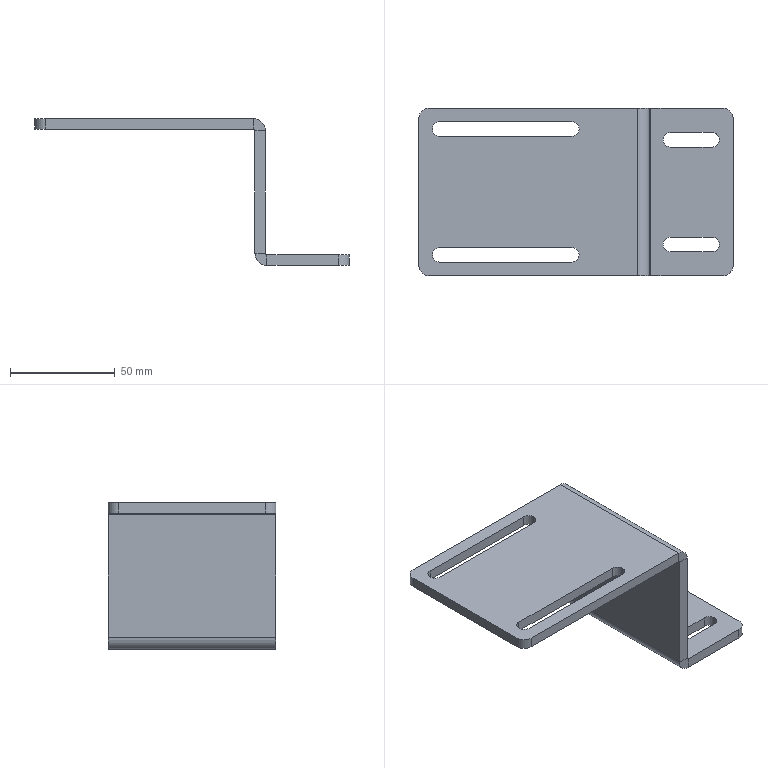Part | SolidWorks | features BaseBody 1 | 1 solid | 46 faces | box 150 x 80 x 70 mm | volume 78202 mm3 | plane 26 | cylinder 20 | commonest cylinder face diameters 7 x12 10 x4 1.473 x2 11.473 x2
STEP:
#1=CARTESIAN_POINT('',(110.,-21.5,-70.));
#2=VERTEX_POINT('',#1);
#3=CARTESIAN_POINT('',(113.5,-25.,-70.));
#4=VERTEX_POINT('',#3);
#5=CARTESIAN_POINT('',(110.,-25.,-70.));
#6=DIRECTION('',(0.,0.,-1.));
#7=DIRECTION('',(-1.,0.,0.));
#8=AXIS2_PLACEMENT_3D('',#5,#6,#7);
#9=CIRCLE('',#8,3.5);
#10=EDGE_CURVE('',#2,#4,#9,.T.);
#11=ORIENTED_EDGE('',*,*,#10,.T.);
#12=CARTESIAN_POINT('',(113.5,-25.,-65.));
#13=VERTEX_POINT('',#12);
#14=CARTESIAN_POINT('',(113.5,-25.,-75.));
#15=DIRECTION('',(0.,0.,1.));
#16=VECTOR('',#15,1000.);
#17=LINE('',#14,#16);
#18=EDGE_CURVE('',#4,#13,#17,.T.);
#19=ORIENTED_EDGE('',*,*,#18,.T.);
#20=CARTESIAN_POINT('',(110.,-21.5,-65.));
#21=VERTEX_POINT('',#20);
#22=CARTESIAN_POINT('',(110.,-25.,-65.));
#23=DIRECTION('',(0.,0.,1.));
#24=DIRECTION('',(1.,0.,0.));
#25=AXIS2_PLACEMENT_3D('',#22,#23,#24);
#26=CIRCLE('',#25,3.5);
#27=EDGE_CURVE('',#13,#21,#26,.T.);
#28=ORIENTED_EDGE('',*,*,#27,.T.);
#29=CARTESIAN_POINT('',(110.,-21.5,-75.));
#30=DIRECTION('',(0.,0.,1.));
#31=VECTOR('',#30,1000.);
#32=LINE('',#29,#31);
#33=EDGE_CURVE('',#2,#21,#32,.T.);
#34=ORIENTED_EDGE('',*,*,#33,.F.);
#35=EDGE_LOOP('',(#11,#19,#28,#34));
#36=FACE_OUTER_BOUND('',#35,.T.);
#37=CARTESIAN_POINT('',(110.,-25.,-75.));
#38=DIRECTION('',(0.,0.,1.));
#39=DIRECTION('',(1.,0.,0.));
#40=AXIS2_PLACEMENT_3D('',#37,#38,#39);
#41=CYLINDRICAL_SURFACE('',#40,3.5);
#42=ADVANCED_FACE('',(#36),#41,.F.);
#43=CARTESIAN_POINT('',(110.,28.5,-70.));
#44=VERTEX_POINT('',#43);
#45=CARTESIAN_POINT('',(113.5,25.,-70.));
#46=VERTEX_POINT('',#45);
#47=CARTESIAN_POINT('',(110.,25.,-70.));
#48=DIRECTION('',(0.,0.,-1.));
#49=DIRECTION('',(-1.,0.,0.));
#50=AXIS2_PLACEMENT_3D('',#47,#48,#49);
#51=CIRCLE('',#50,3.5);
#52=EDGE_CURVE('',#44,#46,#51,.T.);
#53=ORIENTED_EDGE('',*,*,#52,.T.);
#54=CARTESIAN_POINT('',(113.5,25.,-65.));
#55=VERTEX_POINT('',#54);
#56=CARTESIAN_POINT('',(113.5,25.,-75.));
#57=DIRECTION('',(0.,0.,1.));
#58=VECTOR('',#57,1000.);
#59=LINE('',#56,#58);
#60=EDGE_CURVE('',#46,#55,#59,.T.);
#61=ORIENTED_EDGE('',*,*,#60,.T.);
#62=CARTESIAN_POINT('',(110.,28.5,-65.));
#63=VERTEX_POINT('',#62);
#64=CARTESIAN_POINT('',(110.,25.,-65.));
#65=DIRECTION('',(0.,0.,1.));
#66=DIRECTION('',(1.,0.,0.));
#67=AXIS2_PLACEMENT_3D('',#64,#65,#66);
#68=CIRCLE('',#67,3.5);
#69=EDGE_CURVE('',#55,#63,#68,.T.);
#70=ORIENTED_EDGE('',*,*,#69,.T.);
#71=CARTESIAN_POINT('',(110.,28.5,-75.));
#72=DIRECTION('',(0.,0.,1.));
#73=VECTOR('',#72,1000.);
#74=LINE('',#71,#73);
#75=EDGE_CURVE('',#44,#63,#74,.T.);
#76=ORIENTED_EDGE('',*,*,#75,.F.);
#77=EDGE_LOOP('',(#53,#61,#70,#76));
#78=FACE_OUTER_BOUND('',#77,.T.);
#79=CARTESIAN_POINT('',(110.,25.,-75.));
#80=DIRECTION('',(0.,0.,1.));
#81=DIRECTION('',(1.,0.,0.));
#82=AXIS2_PLACEMENT_3D('',#79,#80,#81);
#83=CYLINDRICAL_SURFACE('',#82,3.5);
#84=ADVANCED_FACE('',(#78),#83,.F.);
#85=CARTESIAN_POINT('',(46.5,-30.,-5.));
#86=VERTEX_POINT('',#85);
#87=CARTESIAN_POINT('',(43.,-26.5,-5.));
#88=VERTEX_POINT('',#87);
#89=CARTESIAN_POINT('',(43.,-30.,-5.));
#90=DIRECTION('',(0.,0.,1.));
#91=DIRECTION('',(1.,0.,0.));
#92=AXIS2_PLACEMENT_3D('',#89,#90,#91);
#93=CIRCLE('',#92,3.5);
#94=EDGE_CURVE('',#86,#88,#93,.T.);
#95=ORIENTED_EDGE('',*,*,#94,.F.);
#96=CARTESIAN_POINT('',(46.5,-30.,0.));
#97=VERTEX_POINT('',#96);
#98=CARTESIAN_POINT('',(46.5,-30.,-10.));
#99=DIRECTION('',(0.,0.,1.));
#100=VECTOR('',#99,1000.);
#101=LINE('',#98,#100);
#102=EDGE_CURVE('',#86,#97,#101,.T.);
#103=ORIENTED_EDGE('',*,*,#102,.T.);
#104=CARTESIAN_POINT('',(43.,-26.5,0.));
#105=VERTEX_POINT('',#104);
#106=CARTESIAN_POINT('',(43.,-30.,0.));
#107=DIRECTION('',(0.,0.,1.));
#108=DIRECTION('',(1.,0.,0.));
#109=AXIS2_PLACEMENT_3D('',#106,#107,#108);
#110=CIRCLE('',#109,3.5);
#111=EDGE_CURVE('',#97,#105,#110,.T.);
#112=ORIENTED_EDGE('',*,*,#111,.T.);
#113=CARTESIAN_POINT('',(43.,-26.5,-10.));
#114=DIRECTION('',(0.,0.,1.));
#115=VECTOR('',#114,1000.);
#116=LINE('',#113,#115);
#117=EDGE_CURVE('',#88,#105,#116,.T.);
#118=ORIENTED_EDGE('',*,*,#117,.F.);
#119=EDGE_LOOP('',(#95,#103,#112,#118));
#120=FACE_OUTER_BOUND('',#119,.T.);
#121=CARTESIAN_POINT('',(43.,-30.,-10.));
#122=DIRECTION('',(0.,0.,1.));
#123=DIRECTION('',(1.,0.,0.));
#124=AXIS2_PLACEMENT_3D('',#121,#122,#123);
#125=CYLINDRICAL_SURFACE('',#124,3.5);
#126=ADVANCED_FACE('',(#120),#125,.F.);
#127=CARTESIAN_POINT('',(46.5,30.,-5.));
#128=VERTEX_POINT('',#127);
#129=CARTESIAN_POINT('',(43.,33.5,-5.));
#130=VERTEX_POINT('',#129);
#131=CARTESIAN_POINT('',(43.,30.,-5.));
#132=DIRECTION('',(0.,0.,1.));
#133=DIRECTION('',(1.,0.,0.));
#134=AXIS2_PLACEMENT_3D('',#131,#132,#133);
#135=CIRCLE('',#134,3.5);
#136=EDGE_CURVE('',#128,#130,#135,.T.);
#137=ORIENTED_EDGE('',*,*,#136,.F.);
#138=CARTESIAN_POINT('',(46.5,30.,0.));
#139=VERTEX_POINT('',#138);
#140=CARTESIAN_POINT('',(46.5,30.,-10.));
#141=DIRECTION('',(0.,0.,1.));
#142=VECTOR('',#141,1000.);
#143=LINE('',#140,#142);
#144=EDGE_CURVE('',#128,#139,#143,.T.);
#145=ORIENTED_EDGE('',*,*,#144,.T.);
#146=CARTESIAN_POINT('',(43.,33.5,0.));
#147=VERTEX_POINT('',#146);
#148=CARTESIAN_POINT('',(43.,30.,0.));
#149=DIRECTION('',(0.,0.,1.));
#150=DIRECTION('',(1.,0.,0.));
#151=AXIS2_PLACEMENT_3D('',#148,#149,#150);
#152=CIRCLE('',#151,3.5);
#153=EDGE_CURVE('',#139,#147,#152,.T.);
#154=ORIENTED_EDGE('',*,*,#153,.T.);
#155=CARTESIAN_POINT('',(43.,33.5,-10.));
#156=DIRECTION('',(0.,0.,1.));
#157=VECTOR('',#156,1000.);
#158=LINE('',#155,#157);
#159=EDGE_CURVE('',#130,#147,#158,.T.);
#160=ORIENTED_EDGE('',*,*,#159,.F.);
#161=EDGE_LOOP('',(#137,#145,#154,#160));
#162=FACE_OUTER_BOUND('',#161,.T.);
#163=CARTESIAN_POINT('',(43.,30.,-10.));
#164=DIRECTION('',(0.,0.,1.));
#165=DIRECTION('',(1.,0.,0.));
#166=AXIS2_PLACEMENT_3D('',#163,#164,#165);
#167=CYLINDRICAL_SURFACE('',#166,3.5);
#168=ADVANCED_FACE('',(#162),#167,.F.);
#169=CARTESIAN_POINT('',(80.,40.,-5.737));
#170=VERTEX_POINT('',#169);
#171=CARTESIAN_POINT('',(80.,40.,-64.263));
#172=VERTEX_POINT('',#171);
#173=CARTESIAN_POINT('',(80.,40.,-65.));
#174=DIRECTION('',(0.,0.,-1.));
#175=VECTOR('',#174,1000.);
#176=LINE('',#173,#175);
#177=EDGE_CURVE('',#170,#172,#176,.T.);
#178=ORIENTED_EDGE('',*,*,#177,.T.);
#179=CARTESIAN_POINT('',(75.,40.,-64.263));
#180=VERTEX_POINT('',#179);
#181=CARTESIAN_POINT('',(80.,40.,-64.263));
#182=DIRECTION('',(-1.,0.,0.));
#183=VECTOR('',#182,1000.);
#184=LINE('',#181,#183);
#185=EDGE_CURVE('',#172,#180,#184,.T.);
#186=ORIENTED_EDGE('',*,*,#185,.T.);
#187=CARTESIAN_POINT('',(75.,40.,-5.737));
#188=VERTEX_POINT('',#187);
#189=CARTESIAN_POINT('',(75.,40.,-65.));
#190=DIRECTION('',(0.,0.,-1.));
#191=VECTOR('',#190,1000.);
#192=LINE('',#189,#191);
#193=EDGE_CURVE('',#188,#180,#192,.T.);
#194=ORIENTED_EDGE('',*,*,#193,.F.);
#195=CARTESIAN_POINT('',(75.,40.,-5.737));
#196=DIRECTION('',(1.,0.,0.));
#197=VECTOR('',#196,1000.);
#198=LINE('',#195,#197);
#199=EDGE_CURVE('',#188,#170,#198,.T.);
#200=ORIENTED_EDGE('',*,*,#199,.T.);
#201=EDGE_LOOP('',(#178,#186,#194,#200));
#202=FACE_OUTER_BOUND('',#201,.T.);
#203=CARTESIAN_POINT('',(80.,40.,-65.));
#204=DIRECTION('',(0.,1.,0.));
#205=DIRECTION('',(0.,0.,1.));
#206=AXIS2_PLACEMENT_3D('',#203,#204,#205);
#207=PLANE('',#206);
#208=ADVANCED_FACE('',(#202),#207,.T.);
#209=CARTESIAN_POINT('',(80.,-40.,-64.263));
#210=VERTEX_POINT('',#209);
#211=CARTESIAN_POINT('',(80.,-40.,-5.737));
#212=VERTEX_POINT('',#211);
#213=CARTESIAN_POINT('',(80.,-40.,-5.));
#214=DIRECTION('',(0.,0.,1.));
#215=VECTOR('',#214,1000.);
#216=LINE('',#213,#215);
#217=EDGE_CURVE('',#210,#212,#216,.T.);
#218=ORIENTED_EDGE('',*,*,#217,.F.);
#219=CARTESIAN_POINT('',(80.,40.,-64.263));
#220=DIRECTION('',(0.,-1.,0.));
#221=VECTOR('',#220,1000.);
#222=LINE('',#219,#221);
#223=EDGE_CURVE('',#172,#210,#222,.T.);
#224=ORIENTED_EDGE('',*,*,#223,.F.);
#225=ORIENTED_EDGE('',*,*,#177,.F.);
#226=CARTESIAN_POINT('',(80.,0.,-5.737));
#227=DIRECTION('',(0.,-1.,0.));
#228=VECTOR('',#227,1000.);
#229=LINE('',#226,#228);
#230=EDGE_CURVE('',#170,#212,#229,.T.);
#231=ORIENTED_EDGE('',*,*,#230,.T.);
#232=EDGE_LOOP('',(#218,#224,#225,#231));
#233=FACE_OUTER_BOUND('',#232,.T.);
#234=CARTESIAN_POINT('',(80.,0.,0.));
#235=DIRECTION('',(1.,0.,0.));
#236=DIRECTION('',(0.,0.,-1.));
#237=AXIS2_PLACEMENT_3D('',#234,#235,#236);
#238=PLANE('',#237);
#239=ADVANCED_FACE('',(#233),#238,.T.);
#240=CARTESIAN_POINT('',(75.,-40.,-64.263));
#241=VERTEX_POINT('',#240);
#242=CARTESIAN_POINT('',(75.,40.,-64.263));
#243=DIRECTION('',(0.,-1.,0.));
#244=VECTOR('',#243,1000.);
#245=LINE('',#242,#244);
#246=EDGE_CURVE('',#180,#241,#245,.T.);
#247=ORIENTED_EDGE('',*,*,#246,.T.);
#248=CARTESIAN_POINT('',(75.,-40.,-5.737));
#249=VERTEX_POINT('',#248);
#250=CARTESIAN_POINT('',(75.,-40.,-5.));
#251=DIRECTION('',(0.,0.,1.));
#252=VECTOR('',#251,1000.);
#253=LINE('',#250,#252);
#254=EDGE_CURVE('',#241,#249,#253,.T.);
#255=ORIENTED_EDGE('',*,*,#254,.T.);
#256=CARTESIAN_POINT('',(75.,40.,-5.737));
#257=DIRECTION('',(0.,-1.,0.));
#258=VECTOR('',#257,1000.);
#259=LINE('',#256,#258);
#260=EDGE_CURVE('',#188,#249,#259,.T.);
#261=ORIENTED_EDGE('',*,*,#260,.F.);
#262=ORIENTED_EDGE('',*,*,#193,.T.);
#263=EDGE_LOOP('',(#247,#255,#261,#262));
#264=FACE_OUTER_BOUND('',#263,.T.);
#265=CARTESIAN_POINT('',(75.,0.,0.));
#266=DIRECTION('',(1.,0.,0.));
#267=DIRECTION('',(0.,0.,-1.));
#268=AXIS2_PLACEMENT_3D('',#265,#266,#267);
#269=PLANE('',#268);
#270=ADVANCED_FACE('',(#264),#269,.F.);
#271=CARTESIAN_POINT('',(-25.,-40.,0.));
#272=VERTEX_POINT('',#271);
#273=CARTESIAN_POINT('',(74.263,-40.,0.));
#274=VERTEX_POINT('',#273);
#275=CARTESIAN_POINT('',(-61.,-40.,0.));
#276=DIRECTION('',(1.,0.,0.));
#277=VECTOR('',#276,1000.);
#278=LINE('',#275,#277);
#279=EDGE_CURVE('',#272,#274,#278,.T.);
#280=ORIENTED_EDGE('',*,*,#279,.F.);
#281=CARTESIAN_POINT('',(-25.,-40.,-5.));
#282=VERTEX_POINT('',#281);
#283=CARTESIAN_POINT('',(-25.,-40.,-5.));
#284=DIRECTION('',(0.,0.,-1.));
#285=VECTOR('',#284,1000.);
#286=LINE('',#283,#285);
#287=EDGE_CURVE('',#272,#282,#286,.T.);
#288=ORIENTED_EDGE('',*,*,#287,.T.);
#289=CARTESIAN_POINT('',(74.263,-40.,-5.));
#290=VERTEX_POINT('',#289);
#291=CARTESIAN_POINT('',(-44.,-40.,-5.));
#292=DIRECTION('',(1.,0.,0.));
#293=VECTOR('',#292,1000.);
#294=LINE('',#291,#293);
#295=EDGE_CURVE('',#282,#290,#294,.T.);
#296=ORIENTED_EDGE('',*,*,#295,.T.);
#297=CARTESIAN_POINT('',(74.263,-40.,-5.));
#298=DIRECTION('',(0.,0.,1.));
#299=VECTOR('',#298,1000.);
#300=LINE('',#297,#299);
#301=EDGE_CURVE('',#290,#274,#300,.T.);
#302=ORIENTED_EDGE('',*,*,#301,.T.);
#303=EDGE_LOOP('',(#280,#288,#296,#302));
#304=FACE_OUTER_BOUND('',#303,.T.);
#305=CARTESIAN_POINT('',(-75.,-40.,-5.));
#306=DIRECTION('',(0.,-1.,0.));
#307=DIRECTION('',(0.,0.,-1.));
#308=AXIS2_PLACEMENT_3D('',#305,#306,#307);
#309=PLANE('',#308);
#310=ADVANCED_FACE('',(#304),#309,.T.);
#311=CARTESIAN_POINT('',(-20.,-26.5,-5.));
#312=VERTEX_POINT('',#311);
#313=CARTESIAN_POINT('',(45.,-26.5,-5.));
#314=DIRECTION('',(-1.,0.,0.));
#315=VECTOR('',#314,1000.);
#316=LINE('',#313,#315);
#317=EDGE_CURVE('',#88,#312,#316,.T.);
#318=ORIENTED_EDGE('',*,*,#317,.T.);
#319=CARTESIAN_POINT('',(-20.,-33.5,-5.));
#320=VERTEX_POINT('',#319);
#321=CARTESIAN_POINT('',(-20.,-30.,-5.));
#322=DIRECTION('',(0.,0.,1.));
#323=DIRECTION('',(1.,0.,0.));
#324=AXIS2_PLACEMENT_3D('',#321,#322,#323);
#325=CIRCLE('',#324,3.5);
#326=EDGE_CURVE('',#312,#320,#325,.T.);
#327=ORIENTED_EDGE('',*,*,#326,.T.);
#328=CARTESIAN_POINT('',(43.,-33.5,-5.));
#329=VERTEX_POINT('',#328);
#330=CARTESIAN_POINT('',(45.,-33.5,-5.));
#331=DIRECTION('',(1.,0.,0.));
#332=VECTOR('',#331,1000.);
#333=LINE('',#330,#332);
#334=EDGE_CURVE('',#320,#329,#333,.T.);
#335=ORIENTED_EDGE('',*,*,#334,.T.);
#336=CARTESIAN_POINT('',(43.,-30.,-5.));
#337=DIRECTION('',(0.,0.,1.));
#338=DIRECTION('',(1.,0.,0.));
#339=AXIS2_PLACEMENT_3D('',#336,#337,#338);
#340=CIRCLE('',#339,3.5);
#341=EDGE_CURVE('',#329,#86,#340,.T.);
#342=ORIENTED_EDGE('',*,*,#341,.T.);
#343=ORIENTED_EDGE('',*,*,#94,.T.);
#344=EDGE_LOOP('',(#318,#327,#335,#342,#343));
#345=FACE_BOUND('',#344,.T.);
#346=CARTESIAN_POINT('',(-20.,33.5,-5.));
#347=VERTEX_POINT('',#346);
#348=CARTESIAN_POINT('',(45.,33.5,-5.));
#349=DIRECTION('',(-1.,0.,0.));
#350=VECTOR('',#349,1000.);
#351=LINE('',#348,#350);
#352=EDGE_CURVE('',#130,#347,#351,.T.);
#353=ORIENTED_EDGE('',*,*,#352,.T.);
#354=CARTESIAN_POINT('',(-20.,26.5,-5.));
#355=VERTEX_POINT('',#354);
#356=CARTESIAN_POINT('',(-20.,30.,-5.));
#357=DIRECTION('',(0.,0.,1.));
#358=DIRECTION('',(1.,0.,0.));
#359=AXIS2_PLACEMENT_3D('',#356,#357,#358);
#360=CIRCLE('',#359,3.5);
#361=EDGE_CURVE('',#347,#355,#360,.T.);
#362=ORIENTED_EDGE('',*,*,#361,.T.);
#363=CARTESIAN_POINT('',(43.,26.5,-5.));
#364=VERTEX_POINT('',#363);
#365=CARTESIAN_POINT('',(45.,26.5,-5.));
#366=DIRECTION('',(1.,0.,0.));
#367=VECTOR('',#366,1000.);
#368=LINE('',#365,#367);
#369=EDGE_CURVE('',#355,#364,#368,.T.);
#370=ORIENTED_EDGE('',*,*,#369,.T.);
#371=CARTESIAN_POINT('',(43.,30.,-5.));
#372=DIRECTION('',(0.,0.,1.));
#373=DIRECTION('',(1.,0.,0.));
#374=AXIS2_PLACEMENT_3D('',#371,#372,#373);
#375=CIRCLE('',#374,3.5);
#376=EDGE_CURVE('',#364,#128,#375,.T.);
#377=ORIENTED_EDGE('',*,*,#376,.T.);
#378=ORIENTED_EDGE('',*,*,#136,.T.);
#379=EDGE_LOOP('',(#353,#362,#370,#377,#378));
#380=FACE_BOUND('',#379,.T.);
#381=ORIENTED_EDGE('',*,*,#295,.F.);
#382=CARTESIAN_POINT('',(-30.,-35.,-5.));
#383=VERTEX_POINT('',#382);
#384=CARTESIAN_POINT('',(-25.,-35.,-5.));
#385=DIRECTION('',(0.,0.,-1.));
#386=DIRECTION('',(1.,0.,0.));
#387=AXIS2_PLACEMENT_3D('',#384,#385,#386);
#388=CIRCLE('',#387,5.);
#389=EDGE_CURVE('',#282,#383,#388,.T.);
#390=ORIENTED_EDGE('',*,*,#389,.T.);
#391=CARTESIAN_POINT('',(-30.,35.,-5.));
#392=VERTEX_POINT('',#391);
#393=CARTESIAN_POINT('',(-30.,40.,-5.));
#394=DIRECTION('',(0.,-1.,0.));
#395=VECTOR('',#394,1000.);
#396=LINE('',#393,#395);
#397=EDGE_CURVE('',#392,#383,#396,.T.);
#398=ORIENTED_EDGE('',*,*,#397,.F.);
#399=CARTESIAN_POINT('',(-25.,40.,-5.));
#400=VERTEX_POINT('',#399);
#401=CARTESIAN_POINT('',(-25.,35.,-5.));
#402=DIRECTION('',(0.,0.,-1.));
#403=DIRECTION('',(1.,0.,0.));
#404=AXIS2_PLACEMENT_3D('',#401,#402,#403);
#405=CIRCLE('',#404,5.);
#406=EDGE_CURVE('',#392,#400,#405,.T.);
#407=ORIENTED_EDGE('',*,*,#406,.T.);
#408=CARTESIAN_POINT('',(74.263,40.,-5.));
#409=VERTEX_POINT('',#408);
#410=CARTESIAN_POINT('',(-44.,40.,-5.));
#411=DIRECTION('',(-1.,0.,0.));
#412=VECTOR('',#411,1000.);
#413=LINE('',#410,#412);
#414=EDGE_CURVE('',#409,#400,#413,.T.);
#415=ORIENTED_EDGE('',*,*,#414,.F.);
#416=CARTESIAN_POINT('',(74.263,-40.,-5.));
#417=DIRECTION('',(0.,1.,0.));
#418=VECTOR('',#417,1000.);
#419=LINE('',#416,#418);
#420=EDGE_CURVE('',#290,#409,#419,.T.);
#421=ORIENTED_EDGE('',*,*,#420,.F.);
#422=EDGE_LOOP('',(#381,#390,#398,#407,#415,#421));
#423=FACE_OUTER_BOUND('',#422,.T.);
#424=CARTESIAN_POINT('',(31.,0.,-5.));
#425=DIRECTION('',(0.,0.,1.));
#426=DIRECTION('',(1.,0.,0.));
#427=AXIS2_PLACEMENT_3D('',#424,#425,#426);
#428=PLANE('',#427);
#429=ADVANCED_FACE('',(#345,#380,#423),#428,.F.);
#430=CARTESIAN_POINT('',(-20.,-26.5,0.));
#431=VERTEX_POINT('',#430);
#432=CARTESIAN_POINT('',(-20.,-33.5,0.));
#433=VERTEX_POINT('',#432);
#434=CARTESIAN_POINT('',(-20.,-30.,0.));
#435=DIRECTION('',(0.,0.,1.));
#436=DIRECTION('',(1.,0.,0.));
#437=AXIS2_PLACEMENT_3D('',#434,#435,#436);
#438=CIRCLE('',#437,3.5);
#439=EDGE_CURVE('',#431,#433,#438,.T.);
#440=ORIENTED_EDGE('',*,*,#439,.F.);
#441=CARTESIAN_POINT('',(-20.,-26.5,0.));
#442=DIRECTION('',(-1.,0.,0.));
#443=VECTOR('',#442,1000.);
#444=LINE('',#441,#443);
#445=EDGE_CURVE('',#105,#431,#444,.T.);
#446=ORIENTED_EDGE('',*,*,#445,.F.);
#447=ORIENTED_EDGE('',*,*,#111,.F.);
#448=CARTESIAN_POINT('',(43.,-33.5,0.));
#449=VERTEX_POINT('',#448);
#450=CARTESIAN_POINT('',(43.,-30.,0.));
#451=DIRECTION('',(0.,0.,1.));
#452=DIRECTION('',(1.,0.,0.));
#453=AXIS2_PLACEMENT_3D('',#450,#451,#452);
#454=CIRCLE('',#453,3.5);
#455=EDGE_CURVE('',#449,#97,#454,.T.);
#456=ORIENTED_EDGE('',*,*,#455,.F.);
#457=CARTESIAN_POINT('',(-20.,-33.5,0.));
#458=DIRECTION('',(1.,0.,0.));
#459=VECTOR('',#458,1000.);
#460=LINE('',#457,#459);
#461=EDGE_CURVE('',#433,#449,#460,.T.);
#462=ORIENTED_EDGE('',*,*,#461,.F.);
#463=EDGE_LOOP('',(#440,#446,#447,#456,#462));
#464=FACE_BOUND('',#463,.T.);
#465=CARTESIAN_POINT('',(-20.,33.5,0.));
#466=VERTEX_POINT('',#465);
#467=CARTESIAN_POINT('',(-20.,26.5,0.));
#468=VERTEX_POINT('',#467);
#469=CARTESIAN_POINT('',(-20.,30.,0.));
#470=DIRECTION('',(0.,0.,1.));
#471=DIRECTION('',(1.,0.,0.));
#472=AXIS2_PLACEMENT_3D('',#469,#470,#471);
#473=CIRCLE('',#472,3.5);
#474=EDGE_CURVE('',#466,#468,#473,.T.);
#475=ORIENTED_EDGE('',*,*,#474,.F.);
#476=CARTESIAN_POINT('',(-20.,33.5,0.));
#477=DIRECTION('',(-1.,0.,0.));
#478=VECTOR('',#477,1000.);
#479=LINE('',#476,#478);
#480=EDGE_CURVE('',#147,#466,#479,.T.);
#481=ORIENTED_EDGE('',*,*,#480,.F.);
#482=ORIENTED_EDGE('',*,*,#153,.F.);
#483=CARTESIAN_POINT('',(43.,26.5,0.));
#484=VERTEX_POINT('',#483);
#485=CARTESIAN_POINT('',(43.,30.,0.));
#486=DIRECTION('',(0.,0.,1.));
#487=DIRECTION('',(1.,0.,0.));
#488=AXIS2_PLACEMENT_3D('',#485,#486,#487);
#489=CIRCLE('',#488,3.5);
#490=EDGE_CURVE('',#484,#139,#489,.T.);
#491=ORIENTED_EDGE('',*,*,#490,.F.);
#492=CARTESIAN_POINT('',(-20.,26.5,0.));
#493=DIRECTION('',(1.,0.,0.));
#494=VECTOR('',#493,1000.);
#495=LINE('',#492,#494);
#496=EDGE_CURVE('',#468,#484,#495,.T.);
#497=ORIENTED_EDGE('',*,*,#496,.F.);
#498=EDGE_LOOP('',(#475,#481,#482,#491,#497));
#499=FACE_BOUND('',#498,.T.);
#500=CARTESIAN_POINT('',(-30.,35.,0.));
#501=VERTEX_POINT('',#500);
#502=CARTESIAN_POINT('',(-30.,-35.,0.));
#503=VERTEX_POINT('',#502);
#504=CARTESIAN_POINT('',(-30.,40.,0.));
#505=DIRECTION('',(0.,-1.,0.));
#506=VECTOR('',#505,1000.);
#507=LINE('',#504,#506);
#508=EDGE_CURVE('',#501,#503,#507,.T.);
#509=ORIENTED_EDGE('',*,*,#508,.T.);
#510=CARTESIAN_POINT('',(-25.,-35.,0.));
#511=DIRECTION('',(0.,0.,1.));
#512=DIRECTION('',(1.,0.,0.));
#513=AXIS2_PLACEMENT_3D('',#510,#511,#512);
#514=CIRCLE('',#513,5.);
#515=EDGE_CURVE('',#503,#272,#514,.T.);
#516=ORIENTED_EDGE('',*,*,#515,.T.);
#517=ORIENTED_EDGE('',*,*,#279,.T.);
#518=CARTESIAN_POINT('',(74.263,40.,0.));
#519=VERTEX_POINT('',#518);
#520=CARTESIAN_POINT('',(74.263,-40.,0.));
#521=DIRECTION('',(0.,1.,0.));
#522=VECTOR('',#521,1000.);
#523=LINE('',#520,#522);
#524=EDGE_CURVE('',#274,#519,#523,.T.);
#525=ORIENTED_EDGE('',*,*,#524,.T.);
#526=CARTESIAN_POINT('',(-25.,40.,0.));
#527=VERTEX_POINT('',#526);
#528=CARTESIAN_POINT('',(-61.,40.,0.));
#529=DIRECTION('',(-1.,0.,0.));
#530=VECTOR('',#529,1000.);
#531=LINE('',#528,#530);
#532=EDGE_CURVE('',#519,#527,#531,.T.);
#533=ORIENTED_EDGE('',*,*,#532,.T.);
#534=CARTESIAN_POINT('',(-25.,35.,0.));
#535=DIRECTION('',(0.,0.,1.));
#536=DIRECTION('',(1.,0.,0.));
#537=AXIS2_PLACEMENT_3D('',#534,#535,#536);
#538=CIRCLE('',#537,5.);
#539=EDGE_CURVE('',#527,#501,#538,.T.);
#540=ORIENTED_EDGE('',*,*,#539,.T.);
#541=EDGE_LOOP('',(#509,#516,#517,#525,#533,#540));
#542=FACE_OUTER_BOUND('',#541,.T.);
#543=CARTESIAN_POINT('',(14.,0.,0.));
#544=DIRECTION('',(0.,0.,1.));
#545=DIRECTION('',(1.,0.,0.));
#546=AXIS2_PLACEMENT_3D('',#543,#544,#545);
#547=PLANE('',#546);
#548=ADVANCED_FACE('',(#464,#499,#542),#547,.T.);
#549=ORIENTED_EDGE('',*,*,#397,.T.);
#550=CARTESIAN_POINT('',(-30.,-35.,-5.));
#551=DIRECTION('',(0.,0.,1.));
#552=VECTOR('',#551,1000.);
#553=LINE('',#550,#552);
#554=EDGE_CURVE('',#383,#503,#553,.T.);
#555=ORIENTED_EDGE('',*,*,#554,.T.);
#556=ORIENTED_EDGE('',*,*,#508,.F.);
#557=CARTESIAN_POINT('',(-30.,35.,-5.));
#558=DIRECTION('',(0.,0.,-1.));
#559=VECTOR('',#558,1000.);
#560=LINE('',#557,#559);
#561=EDGE_CURVE('',#501,#392,#560,.T.);
#562=ORIENTED_EDGE('',*,*,#561,.T.);
#563=EDGE_LOOP('',(#549,#555,#556,#562));
#564=FACE_OUTER_BOUND('',#563,.T.);
#565=CARTESIAN_POINT('',(-30.,40.,-5.));
#566=DIRECTION('',(-1.,0.,0.));
#567=DIRECTION('',(0.,-1.,0.));
#568=AXIS2_PLACEMENT_3D('',#565,#566,#567);
#569=PLANE('',#568);
#570=ADVANCED_FACE('',(#564),#569,.T.);
#571=ORIENTED_EDGE('',*,*,#414,.T.);
#572=CARTESIAN_POINT('',(-25.,40.,-5.));
#573=DIRECTION('',(0.,0.,1.));
#574=VECTOR('',#573,1000.);
#575=LINE('',#572,#574);
#576=EDGE_CURVE('',#400,#527,#575,.T.);
#577=ORIENTED_EDGE('',*,*,#576,.T.);
#578=ORIENTED_EDGE('',*,*,#532,.F.);
#579=CARTESIAN_POINT('',(74.263,40.,-5.));
#580=DIRECTION('',(0.,0.,1.));
#581=VECTOR('',#580,1000.);
#582=LINE('',#579,#581);
#583=EDGE_CURVE('',#409,#519,#582,.T.);
#584=ORIENTED_EDGE('',*,*,#583,.F.);
#585=EDGE_LOOP('',(#571,#577,#578,#584));
#586=FACE_OUTER_BOUND('',#585,.T.);
#587=CARTESIAN_POINT('',(-75.,40.,-5.));
#588=DIRECTION('',(0.,1.,0.));
#589=DIRECTION('',(0.,0.,1.));
#590=AXIS2_PLACEMENT_3D('',#587,#588,#589);
#591=PLANE('',#590);
#592=ADVANCED_FACE('',(#586),#591,.T.);
#593=ORIENTED_EDGE('',*,*,#199,.F.);
#594=CARTESIAN_POINT('',(74.263,40.,-5.737));
#595=DIRECTION('',(0.,1.,0.));
#596=DIRECTION('',(0.,0.,-1.));
#597=AXIS2_PLACEMENT_3D('',#594,#595,#596);
#598=CIRCLE('',#597,0.7366);
#599=EDGE_CURVE('',#409,#188,#598,.T.);
#600=ORIENTED_EDGE('',*,*,#599,.F.);
#601=ORIENTED_EDGE('',*,*,#583,.T.);
#602=CARTESIAN_POINT('',(74.263,40.,-5.737));
#603=DIRECTION('',(0.,1.,0.));
#604=DIRECTION('',(0.,0.,-1.));
#605=AXIS2_PLACEMENT_3D('',#602,#603,#604);
#606=CIRCLE('',#605,5.737);
#607=EDGE_CURVE('',#519,#170,#606,.T.);
#608=ORIENTED_EDGE('',*,*,#607,.T.);
#609=EDGE_LOOP('',(#593,#600,#601,#608));
#610=FACE_OUTER_BOUND('',#609,.T.);
#611=CARTESIAN_POINT('',(74.263,40.,-5.737));
#612=DIRECTION('',(0.,1.,0.));
#613=DIRECTION('',(0.,0.,1.));
#614=AXIS2_PLACEMENT_3D('',#611,#612,#613);
#615=PLANE('',#614);
#616=ADVANCED_FACE('',(#610),#615,.T.);
#617=CARTESIAN_POINT('',(74.263,-40.,-5.737));
#618=DIRECTION('',(0.,-1.,0.));
#619=DIRECTION('',(0.,0.,-1.));
#620=AXIS2_PLACEMENT_3D('',#617,#618,#619);
#621=CIRCLE('',#620,0.7366);
#622=EDGE_CURVE('',#249,#290,#621,.T.);
#623=ORIENTED_EDGE('',*,*,#622,.F.);
#624=CARTESIAN_POINT('',(75.,-40.,-5.737));
#625=DIRECTION('',(1.,0.,0.));
#626=VECTOR('',#625,1000.);
#627=LINE('',#624,#626);
#628=EDGE_CURVE('',#249,#212,#627,.T.);
#629=ORIENTED_EDGE('',*,*,#628,.T.);
#630=CARTESIAN_POINT('',(74.263,-40.,-5.737));
#631=DIRECTION('',(0.,-1.,0.));
#632=DIRECTION('',(0.,0.,-1.));
#633=AXIS2_PLACEMENT_3D('',#630,#631,#632);
#634=CIRCLE('',#633,5.737);
#635=EDGE_CURVE('',#212,#274,#634,.T.);
#636=ORIENTED_EDGE('',*,*,#635,.T.);
#637=ORIENTED_EDGE('',*,*,#301,.F.);
#638=EDGE_LOOP('',(#623,#629,#636,#637));
#639=FACE_OUTER_BOUND('',#638,.T.);
#640=CARTESIAN_POINT('',(74.263,-40.,-5.737));
#641=DIRECTION('',(0.,1.,0.));
#642=DIRECTION('',(0.,0.,1.));
#643=AXIS2_PLACEMENT_3D('',#640,#641,#642);
#644=PLANE('',#643);
#645=ADVANCED_FACE('',(#639),#644,.F.);
#646=ORIENTED_EDGE('',*,*,#524,.F.);
#647=ORIENTED_EDGE('',*,*,#635,.F.);
#648=ORIENTED_EDGE('',*,*,#230,.F.);
#649=ORIENTED_EDGE('',*,*,#607,.F.);
#650=EDGE_LOOP('',(#646,#647,#648,#649));
#651=FACE_OUTER_BOUND('',#650,.T.);
#652=CARTESIAN_POINT('',(74.263,-40.,-5.737));
#653=DIRECTION('',(0.,-1.,0.));
#654=DIRECTION('',(1.,0.,0.));
#655=AXIS2_PLACEMENT_3D('',#652,#653,#654);
#656=CYLINDRICAL_SURFACE('',#655,5.737);
#657=ADVANCED_FACE('',(#651),#656,.T.);
#658=ORIENTED_EDGE('',*,*,#420,.T.);
#659=ORIENTED_EDGE('',*,*,#599,.T.);
#660=ORIENTED_EDGE('',*,*,#260,.T.);
#661=ORIENTED_EDGE('',*,*,#622,.T.);
#662=EDGE_LOOP('',(#658,#659,#660,#661));
#663=FACE_OUTER_BOUND('',#662,.T.);
#664=CARTESIAN_POINT('',(74.263,-40.,-5.737));
#665=DIRECTION('',(0.,-1.,0.));
#666=DIRECTION('',(1.,0.,0.));
#667=AXIS2_PLACEMENT_3D('',#664,#665,#666);
#668=CYLINDRICAL_SURFACE('',#667,0.7366);
#669=ADVANCED_FACE('',(#663),#668,.F.);
#670=CARTESIAN_POINT('',(80.,-40.,-64.263));
#671=DIRECTION('',(-1.,0.,0.));
#672=VECTOR('',#671,1000.);
#673=LINE('',#670,#672);
#674=EDGE_CURVE('',#210,#241,#673,.T.);
#675=ORIENTED_EDGE('',*,*,#674,.F.);
#676=ORIENTED_EDGE('',*,*,#217,.T.);
#677=ORIENTED_EDGE('',*,*,#628,.F.);
#678=ORIENTED_EDGE('',*,*,#254,.F.);
#679=EDGE_LOOP('',(#675,#676,#677,#678));
#680=FACE_OUTER_BOUND('',#679,.T.);
#681=CARTESIAN_POINT('',(80.,-40.,-5.));
#682=DIRECTION('',(0.,-1.,0.));
#683=DIRECTION('',(0.,0.,-1.));
#684=AXIS2_PLACEMENT_3D('',#681,#682,#683);
#685=PLANE('',#684);
#686=ADVANCED_FACE('',(#680),#685,.T.);
#687=CARTESIAN_POINT('',(80.737,-40.,-65.));
#688=VERTEX_POINT('',#687);
#689=CARTESIAN_POINT('',(80.737,-40.,-70.));
#690=VERTEX_POINT('',#689);
#691=CARTESIAN_POINT('',(80.737,-40.,-65.));
#692=DIRECTION('',(0.,0.,-1.));
#693=VECTOR('',#692,1000.);
#694=LINE('',#691,#693);
#695=EDGE_CURVE('',#688,#690,#694,.T.);
#696=ORIENTED_EDGE('',*,*,#695,.F.);
#697=CARTESIAN_POINT('',(80.737,-40.,-64.263));
#698=DIRECTION('',(0.,-1.,0.));
#699=DIRECTION('',(0.,0.,1.));
#700=AXIS2_PLACEMENT_3D('',#697,#698,#699);
#701=CIRCLE('',#700,0.7366);
#702=EDGE_CURVE('',#210,#688,#701,.T.);
#703=ORIENTED_EDGE('',*,*,#702,.F.);
#704=ORIENTED_EDGE('',*,*,#674,.T.);
#705=CARTESIAN_POINT('',(80.737,-40.,-64.263));
#706=DIRECTION('',(0.,-1.,0.));
#707=DIRECTION('',(0.,0.,1.));
#708=AXIS2_PLACEMENT_3D('',#705,#706,#707);
#709=CIRCLE('',#708,5.737);
#710=EDGE_CURVE('',#241,#690,#709,.T.);
#711=ORIENTED_EDGE('',*,*,#710,.T.);
#712=EDGE_LOOP('',(#696,#703,#704,#711));
#713=FACE_OUTER_BOUND('',#712,.T.);
#714=CARTESIAN_POINT('',(80.737,-40.,-64.263));
#715=DIRECTION('',(0.,-1.,0.));
#716=DIRECTION('',(0.,0.,-1.));
#717=AXIS2_PLACEMENT_3D('',#714,#715,#716);
#718=PLANE('',#717);
#719=ADVANCED_FACE('',(#713),#718,.T.);
#720=CARTESIAN_POINT('',(80.737,40.,-65.));
#721=VERTEX_POINT('',#720);
#722=CARTESIAN_POINT('',(80.737,40.,-64.263));
#723=DIRECTION('',(0.,1.,0.));
#724=DIRECTION('',(0.,0.,1.));
#725=AXIS2_PLACEMENT_3D('',#722,#723,#724);
#726=CIRCLE('',#725,0.7366);
#727=EDGE_CURVE('',#721,#172,#726,.T.);
#728=ORIENTED_EDGE('',*,*,#727,.F.);
#729=CARTESIAN_POINT('',(80.737,40.,-70.));
#730=VERTEX_POINT('',#729);
#731=CARTESIAN_POINT('',(80.737,40.,-65.));
#732=DIRECTION('',(0.,0.,-1.));
#733=VECTOR('',#732,1000.);
#734=LINE('',#731,#733);
#735=EDGE_CURVE('',#721,#730,#734,.T.);
#736=ORIENTED_EDGE('',*,*,#735,.T.);
#737=CARTESIAN_POINT('',(80.737,40.,-64.263));
#738=DIRECTION('',(0.,1.,0.));
#739=DIRECTION('',(0.,0.,1.));
#740=AXIS2_PLACEMENT_3D('',#737,#738,#739);
#741=CIRCLE('',#740,5.737);
#742=EDGE_CURVE('',#730,#180,#741,.T.);
#743=ORIENTED_EDGE('',*,*,#742,.T.);
#744=ORIENTED_EDGE('',*,*,#185,.F.);
#745=EDGE_LOOP('',(#728,#736,#743,#744));
#746=FACE_OUTER_BOUND('',#745,.T.);
#747=CARTESIAN_POINT('',(80.737,40.,-64.263));
#748=DIRECTION('',(0.,-1.,0.));
#749=DIRECTION('',(0.,0.,-1.));
#750=AXIS2_PLACEMENT_3D('',#747,#748,#749);
#751=PLANE('',#750);
#752=ADVANCED_FACE('',(#746),#751,.F.);
#753=ORIENTED_EDGE('',*,*,#246,.F.);
#754=ORIENTED_EDGE('',*,*,#742,.F.);
#755=CARTESIAN_POINT('',(80.737,0.,-70.));
#756=DIRECTION('',(0.,1.,0.));
#757=VECTOR('',#756,1000.);
#758=LINE('',#755,#757);
#759=EDGE_CURVE('',#690,#730,#758,.T.);
#760=ORIENTED_EDGE('',*,*,#759,.F.);
#761=ORIENTED_EDGE('',*,*,#710,.F.);
#762=EDGE_LOOP('',(#753,#754,#760,#761));
#763=FACE_OUTER_BOUND('',#762,.T.);
#764=CARTESIAN_POINT('',(80.737,40.,-64.263));
#765=DIRECTION('',(0.,1.,0.));
#766=DIRECTION('',(0.,0.,-1.));
#767=AXIS2_PLACEMENT_3D('',#764,#765,#766);
#768=CYLINDRICAL_SURFACE('',#767,5.737);
#769=ADVANCED_FACE('',(#763),#768,.T.);
#770=ORIENTED_EDGE('',*,*,#223,.T.);
#771=ORIENTED_EDGE('',*,*,#702,.T.);
#772=CARTESIAN_POINT('',(80.737,-40.,-65.));
#773=DIRECTION('',(0.,1.,0.));
#774=VECTOR('',#773,1000.);
#775=LINE('',#772,#774);
#776=EDGE_CURVE('',#688,#721,#775,.T.);
#777=ORIENTED_EDGE('',*,*,#776,.T.);
#778=ORIENTED_EDGE('',*,*,#727,.T.);
#779=EDGE_LOOP('',(#770,#771,#777,#778));
#780=FACE_OUTER_BOUND('',#779,.T.);
#781=CARTESIAN_POINT('',(80.737,40.,-64.263));
#782=DIRECTION('',(0.,1.,0.));
#783=DIRECTION('',(0.,0.,-1.));
#784=AXIS2_PLACEMENT_3D('',#781,#782,#783);
#785=CYLINDRICAL_SURFACE('',#784,0.7366);
#786=ADVANCED_FACE('',(#780),#785,.F.);
#787=CARTESIAN_POINT('',(115.,40.,-65.));
#788=VERTEX_POINT('',#787);
#789=CARTESIAN_POINT('',(80.,40.,-65.));
#790=DIRECTION('',(-1.,0.,0.));
#791=VECTOR('',#790,1000.);
#792=LINE('',#789,#791);
#793=EDGE_CURVE('',#788,#721,#792,.T.);
#794=ORIENTED_EDGE('',*,*,#793,.F.);
#795=CARTESIAN_POINT('',(115.,40.,-70.));
#796=VERTEX_POINT('',#795);
#797=CARTESIAN_POINT('',(115.,40.,-70.));
#798=DIRECTION('',(0.,0.,-1.));
#799=VECTOR('',#798,1000.);
#800=LINE('',#797,#799);
#801=EDGE_CURVE('',#788,#796,#800,.T.);
#802=ORIENTED_EDGE('',*,*,#801,.T.);
#803=CARTESIAN_POINT('',(80.,40.,-70.));
#804=DIRECTION('',(-1.,0.,0.));
#805=VECTOR('',#804,1000.);
#806=LINE('',#803,#805);
#807=EDGE_CURVE('',#796,#730,#806,.T.);
#808=ORIENTED_EDGE('',*,*,#807,.T.);
#809=ORIENTED_EDGE('',*,*,#735,.F.);
#810=EDGE_LOOP('',(#794,#802,#808,#809));
#811=FACE_OUTER_BOUND('',#810,.T.);
#812=CARTESIAN_POINT('',(80.,40.,-70.));
#813=DIRECTION('',(0.,1.,0.));
#814=DIRECTION('',(0.,0.,1.));
#815=AXIS2_PLACEMENT_3D('',#812,#813,#814);
#816=PLANE('',#815);
#817=ADVANCED_FACE('',(#811),#816,.T.);
#818=CARTESIAN_POINT('',(115.,-40.,-70.));
#819=VERTEX_POINT('',#818);
#820=CARTESIAN_POINT('',(120.,-40.,-70.));
#821=DIRECTION('',(1.,0.,0.));
#822=VECTOR('',#821,1000.);
#823=LINE('',#820,#822);
#824=EDGE_CURVE('',#690,#819,#823,.T.);
#825=ORIENTED_EDGE('',*,*,#824,.T.);
#826=CARTESIAN_POINT('',(115.,-40.,-65.));
#827=VERTEX_POINT('',#826);
#828=CARTESIAN_POINT('',(115.,-40.,-70.));
#829=DIRECTION('',(0.,0.,1.));
#830=VECTOR('',#829,1000.);
#831=LINE('',#828,#830);
#832=EDGE_CURVE('',#819,#827,#831,.T.);
#833=ORIENTED_EDGE('',*,*,#832,.T.);
#834=CARTESIAN_POINT('',(120.,-40.,-65.));
#835=DIRECTION('',(1.,0.,0.));
#836=VECTOR('',#835,1000.);
#837=LINE('',#834,#836);
#838=EDGE_CURVE('',#688,#827,#837,.T.);
#839=ORIENTED_EDGE('',*,*,#838,.F.);
#840=ORIENTED_EDGE('',*,*,#695,.T.);
#841=EDGE_LOOP('',(#825,#833,#839,#840));
#842=FACE_OUTER_BOUND('',#841,.T.);
#843=CARTESIAN_POINT('',(120.,-40.,-70.));
#844=DIRECTION('',(0.,-1.,0.));
#845=DIRECTION('',(0.,0.,-1.));
#846=AXIS2_PLACEMENT_3D('',#843,#844,#845);
#847=PLANE('',#846);
#848=ADVANCED_FACE('',(#842),#847,.T.);
#849=CARTESIAN_POINT('',(90.,-28.5,-70.));
#850=VERTEX_POINT('',#849);
#851=CARTESIAN_POINT('',(90.,-21.5,-70.));
#852=VERTEX_POINT('',#851);
#853=CARTESIAN_POINT('',(90.,-25.,-70.));
#854=DIRECTION('',(0.,0.,-1.));
#855=DIRECTION('',(-1.,0.,0.));
#856=AXIS2_PLACEMENT_3D('',#853,#854,#855);
#857=CIRCLE('',#856,3.5);
#858=EDGE_CURVE('',#850,#852,#857,.T.);
#859=ORIENTED_EDGE('',*,*,#858,.F.);
#860=CARTESIAN_POINT('',(110.,-28.5,-70.));
#861=VERTEX_POINT('',#860);
#862=CARTESIAN_POINT('',(0.,-28.5,-70.));
#863=DIRECTION('',(-1.,0.,0.));
#864=VECTOR('',#863,1000.);
#865=LINE('',#862,#864);
#866=EDGE_CURVE('',#861,#850,#865,.T.);
#867=ORIENTED_EDGE('',*,*,#866,.F.);
#868=CARTESIAN_POINT('',(110.,-25.,-70.));
#869=DIRECTION('',(0.,0.,-1.));
#870=DIRECTION('',(-1.,0.,0.));
#871=AXIS2_PLACEMENT_3D('',#868,#869,#870);
#872=CIRCLE('',#871,3.5);
#873=EDGE_CURVE('',#4,#861,#872,.T.);
#874=ORIENTED_EDGE('',*,*,#873,.F.);
#875=ORIENTED_EDGE('',*,*,#10,.F.);
#876=CARTESIAN_POINT('',(0.,-21.5,-70.));
#877=DIRECTION('',(1.,0.,0.));
#878=VECTOR('',#877,1000.);
#879=LINE('',#876,#878);
#880=EDGE_CURVE('',#852,#2,#879,.T.);
#881=ORIENTED_EDGE('',*,*,#880,.F.);
#882=EDGE_LOOP('',(#859,#867,#874,#875,#881));
#883=FACE_BOUND('',#882,.T.);
#884=CARTESIAN_POINT('',(90.,21.5,-70.));
#885=VERTEX_POINT('',#884);
#886=CARTESIAN_POINT('',(90.,28.5,-70.));
#887=VERTEX_POINT('',#886);
#888=CARTESIAN_POINT('',(90.,25.,-70.));
#889=DIRECTION('',(0.,0.,-1.));
#890=DIRECTION('',(-1.,0.,0.));
#891=AXIS2_PLACEMENT_3D('',#888,#889,#890);
#892=CIRCLE('',#891,3.5);
#893=EDGE_CURVE('',#885,#887,#892,.T.);
#894=ORIENTED_EDGE('',*,*,#893,.F.);
#895=CARTESIAN_POINT('',(110.,21.5,-70.));
#896=VERTEX_POINT('',#895);
#897=CARTESIAN_POINT('',(0.,21.5,-70.));
#898=DIRECTION('',(-1.,0.,0.));
#899=VECTOR('',#898,1000.);
#900=LINE('',#897,#899);
#901=EDGE_CURVE('',#896,#885,#900,.T.);
#902=ORIENTED_EDGE('',*,*,#901,.F.);
#903=CARTESIAN_POINT('',(110.,25.,-70.));
#904=DIRECTION('',(0.,0.,-1.));
#905=DIRECTION('',(-1.,0.,0.));
#906=AXIS2_PLACEMENT_3D('',#903,#904,#905);
#907=CIRCLE('',#906,3.5);
#908=EDGE_CURVE('',#46,#896,#907,.T.);
#909=ORIENTED_EDGE('',*,*,#908,.F.);
#910=ORIENTED_EDGE('',*,*,#52,.F.);
#911=CARTESIAN_POINT('',(0.,28.5,-70.));
#912=DIRECTION('',(1.,0.,0.));
#913=VECTOR('',#912,1000.);
#914=LINE('',#911,#913);
#915=EDGE_CURVE('',#887,#44,#914,.T.);
#916=ORIENTED_EDGE('',*,*,#915,.F.);
#917=EDGE_LOOP('',(#894,#902,#909,#910,#916));
#918=FACE_BOUND('',#917,.T.);
#919=CARTESIAN_POINT('',(120.,-35.,-70.));
#920=VERTEX_POINT('',#919);
#921=CARTESIAN_POINT('',(120.,35.,-70.));
#922=VERTEX_POINT('',#921);
#923=CARTESIAN_POINT('',(120.,40.,-70.));
#924=DIRECTION('',(0.,1.,0.));
#925=VECTOR('',#924,1000.);
#926=LINE('',#923,#925);
#927=EDGE_CURVE('',#920,#922,#926,.T.);
#928=ORIENTED_EDGE('',*,*,#927,.F.);
#929=CARTESIAN_POINT('',(115.,-35.,-70.));
#930=DIRECTION('',(0.,0.,-1.));
#931=DIRECTION('',(-1.,0.,0.));
#932=AXIS2_PLACEMENT_3D('',#929,#930,#931);
#933=CIRCLE('',#932,5.);
#934=EDGE_CURVE('',#920,#819,#933,.T.);
#935=ORIENTED_EDGE('',*,*,#934,.T.);
#936=ORIENTED_EDGE('',*,*,#824,.F.);
#937=ORIENTED_EDGE('',*,*,#759,.T.);
#938=ORIENTED_EDGE('',*,*,#807,.F.);
#939=CARTESIAN_POINT('',(115.,35.,-70.));
#940=DIRECTION('',(0.,0.,-1.));
#941=DIRECTION('',(-1.,0.,0.));
#942=AXIS2_PLACEMENT_3D('',#939,#940,#941);
#943=CIRCLE('',#942,5.);
#944=EDGE_CURVE('',#796,#922,#943,.T.);
#945=ORIENTED_EDGE('',*,*,#944,.T.);
#946=EDGE_LOOP('',(#928,#935,#936,#937,#938,#945));
#947=FACE_OUTER_BOUND('',#946,.T.);
#948=CARTESIAN_POINT('',(0.,0.,-70.));
#949=DIRECTION('',(0.,0.,-1.));
#950=DIRECTION('',(-1.,0.,0.));
#951=AXIS2_PLACEMENT_3D('',#948,#949,#950);
#952=PLANE('',#951);
#953=ADVANCED_FACE('',(#883,#918,#947),#952,.T.);
#954=CARTESIAN_POINT('',(90.,-28.5,-65.));
#955=VERTEX_POINT('',#954);
#956=CARTESIAN_POINT('',(110.,-28.5,-65.));
#957=VERTEX_POINT('',#956);
#958=CARTESIAN_POINT('',(90.,-28.5,-65.));
#959=DIRECTION('',(1.,0.,0.));
#960=VECTOR('',#959,1000.);
#961=LINE('',#958,#960);
#962=EDGE_CURVE('',#955,#957,#961,.T.);
#963=ORIENTED_EDGE('',*,*,#962,.F.);
#964=CARTESIAN_POINT('',(90.,-21.5,-65.));
#965=VERTEX_POINT('',#964);
#966=CARTESIAN_POINT('',(90.,-25.,-65.));
#967=DIRECTION('',(0.,0.,1.));
#968=DIRECTION('',(1.,0.,0.));
#969=AXIS2_PLACEMENT_3D('',#966,#967,#968);
#970=CIRCLE('',#969,3.5);
#971=EDGE_CURVE('',#965,#955,#970,.T.);
#972=ORIENTED_EDGE('',*,*,#971,.F.);
#973=CARTESIAN_POINT('',(90.,-21.5,-65.));
#974=DIRECTION('',(-1.,0.,0.));
#975=VECTOR('',#974,1000.);
#976=LINE('',#973,#975);
#977=EDGE_CURVE('',#21,#965,#976,.T.);
#978=ORIENTED_EDGE('',*,*,#977,.F.);
#979=ORIENTED_EDGE('',*,*,#27,.F.);
#980=CARTESIAN_POINT('',(110.,-25.,-65.));
#981=DIRECTION('',(0.,0.,1.));
#982=DIRECTION('',(1.,0.,0.));
#983=AXIS2_PLACEMENT_3D('',#980,#981,#982);
#984=CIRCLE('',#983,3.5);
#985=EDGE_CURVE('',#957,#13,#984,.T.);
#986=ORIENTED_EDGE('',*,*,#985,.F.);
#987=EDGE_LOOP('',(#963,#972,#978,#979,#986));
#988=FACE_BOUND('',#987,.T.);
#989=CARTESIAN_POINT('',(90.,21.5,-65.));
#990=VERTEX_POINT('',#989);
#991=CARTESIAN_POINT('',(110.,21.5,-65.));
#992=VERTEX_POINT('',#991);
#993=CARTESIAN_POINT('',(90.,21.5,-65.));
#994=DIRECTION('',(1.,0.,0.));
#995=VECTOR('',#994,1000.);
#996=LINE('',#993,#995);
#997=EDGE_CURVE('',#990,#992,#996,.T.);
#998=ORIENTED_EDGE('',*,*,#997,.F.);
#999=CARTESIAN_POINT('',(90.,28.5,-65.));
#1000=VERTEX_POINT('',#999);
#1001=CARTESIAN_POINT('',(90.,25.,-65.));
#1002=DIRECTION('',(0.,0.,1.));
#1003=DIRECTION('',(1.,0.,0.));
#1004=AXIS2_PLACEMENT_3D('',#1001,#1002,#1003);
#1005=CIRCLE('',#1004,3.5);
#1006=EDGE_CURVE('',#1000,#990,#1005,.T.);
#1007=ORIENTED_EDGE('',*,*,#1006,.F.);
#1008=CARTESIAN_POINT('',(90.,28.5,-65.));
#1009=DIRECTION('',(-1.,0.,0.));
#1010=VECTOR('',#1009,1000.);
#1011=LINE('',#1008,#1010);
#1012=EDGE_CURVE('',#63,#1000,#1011,.T.);
#1013=ORIENTED_EDGE('',*,*,#1012,.F.);
#1014=ORIENTED_EDGE('',*,*,#69,.F.);
#1015=CARTESIAN_POINT('',(110.,25.,-65.));
#1016=DIRECTION('',(0.,0.,1.));
#1017=DIRECTION('',(1.,0.,0.));
#1018=AXIS2_PLACEMENT_3D('',#1015,#1016,#1017);
#1019=CIRCLE('',#1018,3.5);
#1020=EDGE_CURVE('',#992,#55,#1019,.T.);
#1021=ORIENTED_EDGE('',*,*,#1020,.F.);
#1022=EDGE_LOOP('',(#998,#1007,#1013,#1014,#1021));
#1023=FACE_BOUND('',#1022,.T.);
#1024=ORIENTED_EDGE('',*,*,#838,.T.);
#1025=CARTESIAN_POINT('',(120.,-35.,-65.));
#1026=VERTEX_POINT('',#1025);
#1027=CARTESIAN_POINT('',(115.,-35.,-65.));
#1028=DIRECTION('',(0.,0.,1.));
#1029=DIRECTION('',(-1.,0.,0.));
#1030=AXIS2_PLACEMENT_3D('',#1027,#1028,#1029);
#1031=CIRCLE('',#1030,5.);
#1032=EDGE_CURVE('',#827,#1026,#1031,.T.);
#1033=ORIENTED_EDGE('',*,*,#1032,.T.);
#1034=CARTESIAN_POINT('',(120.,35.,-65.));
#1035=VERTEX_POINT('',#1034);
#1036=CARTESIAN_POINT('',(120.,40.,-65.));
#1037=DIRECTION('',(0.,1.,0.));
#1038=VECTOR('',#1037,1000.);
#1039=LINE('',#1036,#1038);
#1040=EDGE_CURVE('',#1026,#1035,#1039,.T.);
#1041=ORIENTED_EDGE('',*,*,#1040,.T.);
#1042=CARTESIAN_POINT('',(115.,35.,-65.));
#1043=DIRECTION('',(0.,0.,1.));
#1044=DIRECTION('',(-1.,0.,0.));
#1045=AXIS2_PLACEMENT_3D('',#1042,#1043,#1044);
#1046=CIRCLE('',#1045,5.);
#1047=EDGE_CURVE('',#1035,#788,#1046,.T.);
#1048=ORIENTED_EDGE('',*,*,#1047,.T.);
#1049=ORIENTED_EDGE('',*,*,#793,.T.);
#1050=ORIENTED_EDGE('',*,*,#776,.F.);
#1051=EDGE_LOOP('',(#1024,#1033,#1041,#1048,#1049,#1050));
#1052=FACE_OUTER_BOUND('',#1051,.T.);
#1053=CARTESIAN_POINT('',(0.,0.,-65.));
#1054=DIRECTION('',(0.,0.,-1.));
#1055=DIRECTION('',(-1.,0.,0.));
#1056=AXIS2_PLACEMENT_3D('',#1053,#1054,#1055);
#1057=PLANE('',#1056);
#1058=ADVANCED_FACE('',(#988,#1023,#1052),#1057,.F.);
#1059=ORIENTED_EDGE('',*,*,#1040,.F.);
#1060=CARTESIAN_POINT('',(120.,-35.,-70.));
#1061=DIRECTION('',(0.,0.,-1.));
#1062=VECTOR('',#1061,1000.);
#1063=LINE('',#1060,#1062);
#1064=EDGE_CURVE('',#1026,#920,#1063,.T.);
#1065=ORIENTED_EDGE('',*,*,#1064,.T.);
#1066=ORIENTED_EDGE('',*,*,#927,.T.);
#1067=CARTESIAN_POINT('',(120.,35.,-70.));
#1068=DIRECTION('',(0.,0.,1.));
#1069=VECTOR('',#1068,1000.);
#1070=LINE('',#1067,#1069);
#1071=EDGE_CURVE('',#922,#1035,#1070,.T.);
#1072=ORIENTED_EDGE('',*,*,#1071,.T.);
#1073=EDGE_LOOP('',(#1059,#1065,#1066,#1072));
#1074=FACE_OUTER_BOUND('',#1073,.T.);
#1075=CARTESIAN_POINT('',(120.,40.,-70.));
#1076=DIRECTION('',(1.,0.,0.));
#1077=DIRECTION('',(0.,0.,-1.));
#1078=AXIS2_PLACEMENT_3D('',#1075,#1076,#1077);
#1079=PLANE('',#1078);
#1080=ADVANCED_FACE('',(#1074),#1079,.T.);
#1081=ORIENTED_EDGE('',*,*,#934,.F.);
#1082=ORIENTED_EDGE('',*,*,#1064,.F.);
#1083=ORIENTED_EDGE('',*,*,#1032,.F.);
#1084=ORIENTED_EDGE('',*,*,#832,.F.);
#1085=EDGE_LOOP('',(#1081,#1082,#1083,#1084));
#1086=FACE_OUTER_BOUND('',#1085,.T.);
#1087=CARTESIAN_POINT('',(115.,-35.,-70.));
#1088=DIRECTION('',(0.,0.,1.));
#1089=DIRECTION('',(1.,0.,0.));
#1090=AXIS2_PLACEMENT_3D('',#1087,#1088,#1089);
#1091=CYLINDRICAL_SURFACE('',#1090,5.);
#1092=ADVANCED_FACE('',(#1086),#1091,.T.);
#1093=ORIENTED_EDGE('',*,*,#944,.F.);
#1094=ORIENTED_EDGE('',*,*,#801,.F.);
#1095=ORIENTED_EDGE('',*,*,#1047,.F.);
#1096=ORIENTED_EDGE('',*,*,#1071,.F.);
#1097=EDGE_LOOP('',(#1093,#1094,#1095,#1096));
#1098=FACE_OUTER_BOUND('',#1097,.T.);
#1099=CARTESIAN_POINT('',(115.,35.,-70.));
#1100=DIRECTION('',(0.,0.,1.));
#1101=DIRECTION('',(1.,0.,0.));
#1102=AXIS2_PLACEMENT_3D('',#1099,#1100,#1101);
#1103=CYLINDRICAL_SURFACE('',#1102,5.);
#1104=ADVANCED_FACE('',(#1098),#1103,.T.);
#1105=ORIENTED_EDGE('',*,*,#389,.F.);
#1106=ORIENTED_EDGE('',*,*,#287,.F.);
#1107=ORIENTED_EDGE('',*,*,#515,.F.);
#1108=ORIENTED_EDGE('',*,*,#554,.F.);
#1109=EDGE_LOOP('',(#1105,#1106,#1107,#1108));
#1110=FACE_OUTER_BOUND('',#1109,.T.);
#1111=CARTESIAN_POINT('',(-25.,-35.,-5.));
#1112=DIRECTION('',(0.,0.,1.));
#1113=DIRECTION('',(1.,0.,0.));
#1114=AXIS2_PLACEMENT_3D('',#1111,#1112,#1113);
#1115=CYLINDRICAL_SURFACE('',#1114,5.);
#1116=ADVANCED_FACE('',(#1110),#1115,.T.);
#1117=ORIENTED_EDGE('',*,*,#406,.F.);
#1118=ORIENTED_EDGE('',*,*,#561,.F.);
#1119=ORIENTED_EDGE('',*,*,#539,.F.);
#1120=ORIENTED_EDGE('',*,*,#576,.F.);
#1121=EDGE_LOOP('',(#1117,#1118,#1119,#1120));
#1122=FACE_OUTER_BOUND('',#1121,.T.);
#1123=CARTESIAN_POINT('',(-25.,35.,-5.));
#1124=DIRECTION('',(0.,0.,1.));
#1125=DIRECTION('',(1.,0.,0.));
#1126=AXIS2_PLACEMENT_3D('',#1123,#1124,#1125);
#1127=CYLINDRICAL_SURFACE('',#1126,5.);
#1128=ADVANCED_FACE('',(#1122),#1127,.T.);
#1129=CARTESIAN_POINT('',(-20.,33.5,-10.));
#1130=DIRECTION('',(0.,0.,1.));
#1131=VECTOR('',#1130,1000.);
#1132=LINE('',#1129,#1131);
#1133=EDGE_CURVE('',#347,#466,#1132,.T.);
#1134=ORIENTED_EDGE('',*,*,#1133,.T.);
#1135=ORIENTED_EDGE('',*,*,#474,.T.);
#1136=CARTESIAN_POINT('',(-20.,26.5,-10.));
#1137=DIRECTION('',(0.,0.,1.));
#1138=VECTOR('',#1137,1000.);
#1139=LINE('',#1136,#1138);
#1140=EDGE_CURVE('',#355,#468,#1139,.T.);
#1141=ORIENTED_EDGE('',*,*,#1140,.F.);
#1142=ORIENTED_EDGE('',*,*,#361,.F.);
#1143=EDGE_LOOP('',(#1134,#1135,#1141,#1142));
#1144=FACE_OUTER_BOUND('',#1143,.T.);
#1145=CARTESIAN_POINT('',(-20.,30.,-10.));
#1146=DIRECTION('',(0.,0.,1.));
#1147=DIRECTION('',(1.,0.,0.));
#1148=AXIS2_PLACEMENT_3D('',#1145,#1146,#1147);
#1149=CYLINDRICAL_SURFACE('',#1148,3.5);
#1150=ADVANCED_FACE('',(#1144),#1149,.F.);
#1151=ORIENTED_EDGE('',*,*,#159,.T.);
#1152=ORIENTED_EDGE('',*,*,#480,.T.);
#1153=ORIENTED_EDGE('',*,*,#1133,.F.);
#1154=ORIENTED_EDGE('',*,*,#352,.F.);
#1155=EDGE_LOOP('',(#1151,#1152,#1153,#1154));
#1156=FACE_OUTER_BOUND('',#1155,.T.);
#1157=CARTESIAN_POINT('',(-20.,33.5,-10.));
#1158=DIRECTION('',(0.,1.,0.));
#1159=DIRECTION('',(-1.,0.,0.));
#1160=AXIS2_PLACEMENT_3D('',#1157,#1158,#1159);
#1161=PLANE('',#1160);
#1162=ADVANCED_FACE('',(#1156),#1161,.F.);
#1163=ORIENTED_EDGE('',*,*,#144,.F.);
#1164=ORIENTED_EDGE('',*,*,#376,.F.);
#1165=CARTESIAN_POINT('',(43.,26.5,-10.));
#1166=DIRECTION('',(0.,0.,1.));
#1167=VECTOR('',#1166,1000.);
#1168=LINE('',#1165,#1167);
#1169=EDGE_CURVE('',#364,#484,#1168,.T.);
#1170=ORIENTED_EDGE('',*,*,#1169,.T.);
#1171=ORIENTED_EDGE('',*,*,#490,.T.);
#1172=EDGE_LOOP('',(#1163,#1164,#1170,#1171));
#1173=FACE_OUTER_BOUND('',#1172,.T.);
#1174=CARTESIAN_POINT('',(43.,30.,-10.));
#1175=DIRECTION('',(0.,0.,1.));
#1176=DIRECTION('',(1.,0.,0.));
#1177=AXIS2_PLACEMENT_3D('',#1174,#1175,#1176);
#1178=CYLINDRICAL_SURFACE('',#1177,3.5);
#1179=ADVANCED_FACE('',(#1173),#1178,.F.);
#1180=ORIENTED_EDGE('',*,*,#1140,.T.);
#1181=ORIENTED_EDGE('',*,*,#496,.T.);
#1182=ORIENTED_EDGE('',*,*,#1169,.F.);
#1183=ORIENTED_EDGE('',*,*,#369,.F.);
#1184=EDGE_LOOP('',(#1180,#1181,#1182,#1183));
#1185=FACE_OUTER_BOUND('',#1184,.T.);
#1186=CARTESIAN_POINT('',(-20.,26.5,-10.));
#1187=DIRECTION('',(0.,-1.,0.));
#1188=DIRECTION('',(1.,0.,0.));
#1189=AXIS2_PLACEMENT_3D('',#1186,#1187,#1188);
#1190=PLANE('',#1189);
#1191=ADVANCED_FACE('',(#1185),#1190,.F.);
#1192=CARTESIAN_POINT('',(-20.,-26.5,-10.));
#1193=DIRECTION('',(0.,0.,1.));
#1194=VECTOR('',#1193,1000.);
#1195=LINE('',#1192,#1194);
#1196=EDGE_CURVE('',#312,#431,#1195,.T.);
#1197=ORIENTED_EDGE('',*,*,#1196,.T.);
#1198=ORIENTED_EDGE('',*,*,#439,.T.);
#1199=CARTESIAN_POINT('',(-20.,-33.5,-10.));
#1200=DIRECTION('',(0.,0.,1.));
#1201=VECTOR('',#1200,1000.);
#1202=LINE('',#1199,#1201);
#1203=EDGE_CURVE('',#320,#433,#1202,.T.);
#1204=ORIENTED_EDGE('',*,*,#1203,.F.);
#1205=ORIENTED_EDGE('',*,*,#326,.F.);
#1206=EDGE_LOOP('',(#1197,#1198,#1204,#1205));
#1207=FACE_OUTER_BOUND('',#1206,.T.);
#1208=CARTESIAN_POINT('',(-20.,-30.,-10.));
#1209=DIRECTION('',(0.,0.,1.));
#1210=DIRECTION('',(1.,0.,0.));
#1211=AXIS2_PLACEMENT_3D('',#1208,#1209,#1210);
#1212=CYLINDRICAL_SURFACE('',#1211,3.5);
#1213=ADVANCED_FACE('',(#1207),#1212,.F.);
#1214=ORIENTED_EDGE('',*,*,#117,.T.);
#1215=ORIENTED_EDGE('',*,*,#445,.T.);
#1216=ORIENTED_EDGE('',*,*,#1196,.F.);
#1217=ORIENTED_EDGE('',*,*,#317,.F.);
#1218=EDGE_LOOP('',(#1214,#1215,#1216,#1217));
#1219=FACE_OUTER_BOUND('',#1218,.T.);
#1220=CARTESIAN_POINT('',(-20.,-26.5,-10.));
#1221=DIRECTION('',(0.,1.,0.));
#1222=DIRECTION('',(0.,0.,1.));
#1223=AXIS2_PLACEMENT_3D('',#1220,#1221,#1222);
#1224=PLANE('',#1223);
#1225=ADVANCED_FACE('',(#1219),#1224,.F.);
#1226=ORIENTED_EDGE('',*,*,#102,.F.);
#1227=ORIENTED_EDGE('',*,*,#341,.F.);
#1228=CARTESIAN_POINT('',(43.,-33.5,-10.));
#1229=DIRECTION('',(0.,0.,1.));
#1230=VECTOR('',#1229,1000.);
#1231=LINE('',#1228,#1230);
#1232=EDGE_CURVE('',#329,#449,#1231,.T.);
#1233=ORIENTED_EDGE('',*,*,#1232,.T.);
#1234=ORIENTED_EDGE('',*,*,#455,.T.);
#1235=EDGE_LOOP('',(#1226,#1227,#1233,#1234));
#1236=FACE_OUTER_BOUND('',#1235,.T.);
#1237=CARTESIAN_POINT('',(43.,-30.,-10.));
#1238=DIRECTION('',(0.,0.,1.));
#1239=DIRECTION('',(1.,0.,0.));
#1240=AXIS2_PLACEMENT_3D('',#1237,#1238,#1239);
#1241=CYLINDRICAL_SURFACE('',#1240,3.5);
#1242=ADVANCED_FACE('',(#1236),#1241,.F.);
#1243=ORIENTED_EDGE('',*,*,#1203,.T.);
#1244=ORIENTED_EDGE('',*,*,#461,.T.);
#1245=ORIENTED_EDGE('',*,*,#1232,.F.);
#1246=ORIENTED_EDGE('',*,*,#334,.F.);
#1247=EDGE_LOOP('',(#1243,#1244,#1245,#1246));
#1248=FACE_OUTER_BOUND('',#1247,.T.);
#1249=CARTESIAN_POINT('',(-20.,-33.5,-10.));
#1250=DIRECTION('',(0.,-1.,0.));
#1251=DIRECTION('',(0.,0.,-1.));
#1252=AXIS2_PLACEMENT_3D('',#1249,#1250,#1251);
#1253=PLANE('',#1252);
#1254=ADVANCED_FACE('',(#1248),#1253,.F.);
#1255=ORIENTED_EDGE('',*,*,#893,.T.);
#1256=CARTESIAN_POINT('',(90.,28.5,-75.));
#1257=DIRECTION('',(0.,0.,1.));
#1258=VECTOR('',#1257,1000.);
#1259=LINE('',#1256,#1258);
#1260=EDGE_CURVE('',#887,#1000,#1259,.T.);
#1261=ORIENTED_EDGE('',*,*,#1260,.T.);
#1262=ORIENTED_EDGE('',*,*,#1006,.T.);
#1263=CARTESIAN_POINT('',(90.,21.5,-75.));
#1264=DIRECTION('',(0.,0.,1.));
#1265=VECTOR('',#1264,1000.);
#1266=LINE('',#1263,#1265);
#1267=EDGE_CURVE('',#885,#990,#1266,.T.);
#1268=ORIENTED_EDGE('',*,*,#1267,.F.);
#1269=EDGE_LOOP('',(#1255,#1261,#1262,#1268));
#1270=FACE_OUTER_BOUND('',#1269,.T.);
#1271=CARTESIAN_POINT('',(90.,25.,-75.));
#1272=DIRECTION('',(0.,0.,1.));
#1273=DIRECTION('',(1.,0.,0.));
#1274=AXIS2_PLACEMENT_3D('',#1271,#1272,#1273);
#1275=CYLINDRICAL_SURFACE('',#1274,3.5);
#1276=ADVANCED_FACE('',(#1270),#1275,.F.);
#1277=ORIENTED_EDGE('',*,*,#915,.T.);
#1278=ORIENTED_EDGE('',*,*,#75,.T.);
#1279=ORIENTED_EDGE('',*,*,#1012,.T.);
#1280=ORIENTED_EDGE('',*,*,#1260,.F.);
#1281=EDGE_LOOP('',(#1277,#1278,#1279,#1280));
#1282=FACE_OUTER_BOUND('',#1281,.T.);
#1283=CARTESIAN_POINT('',(90.,28.5,-75.));
#1284=DIRECTION('',(0.,1.,0.));
#1285=DIRECTION('',(0.,0.,1.));
#1286=AXIS2_PLACEMENT_3D('',#1283,#1284,#1285);
#1287=PLANE('',#1286);
#1288=ADVANCED_FACE('',(#1282),#1287,.F.);
#1289=ORIENTED_EDGE('',*,*,#60,.F.);
#1290=ORIENTED_EDGE('',*,*,#908,.T.);
#1291=CARTESIAN_POINT('',(110.,21.5,-75.));
#1292=DIRECTION('',(0.,0.,1.));
#1293=VECTOR('',#1292,1000.);
#1294=LINE('',#1291,#1293);
#1295=EDGE_CURVE('',#896,#992,#1294,.T.);
#1296=ORIENTED_EDGE('',*,*,#1295,.T.);
#1297=ORIENTED_EDGE('',*,*,#1020,.T.);
#1298=EDGE_LOOP('',(#1289,#1290,#1296,#1297));
#1299=FACE_OUTER_BOUND('',#1298,.T.);
#1300=CARTESIAN_POINT('',(110.,25.,-75.));
#1301=DIRECTION('',(0.,0.,1.));
#1302=DIRECTION('',(1.,0.,0.));
#1303=AXIS2_PLACEMENT_3D('',#1300,#1301,#1302);
#1304=CYLINDRICAL_SURFACE('',#1303,3.5);
#1305=ADVANCED_FACE('',(#1299),#1304,.F.);
#1306=ORIENTED_EDGE('',*,*,#901,.T.);
#1307=ORIENTED_EDGE('',*,*,#1267,.T.);
#1308=ORIENTED_EDGE('',*,*,#997,.T.);
#1309=ORIENTED_EDGE('',*,*,#1295,.F.);
#1310=EDGE_LOOP('',(#1306,#1307,#1308,#1309));
#1311=FACE_OUTER_BOUND('',#1310,.T.);
#1312=CARTESIAN_POINT('',(90.,21.5,-75.));
#1313=DIRECTION('',(0.,-1.,0.));
#1314=DIRECTION('',(1.,0.,0.));
#1315=AXIS2_PLACEMENT_3D('',#1312,#1313,#1314);
#1316=PLANE('',#1315);
#1317=ADVANCED_FACE('',(#1311),#1316,.F.);
#1318=ORIENTED_EDGE('',*,*,#858,.T.);
#1319=CARTESIAN_POINT('',(90.,-21.5,-75.));
#1320=DIRECTION('',(0.,0.,1.));
#1321=VECTOR('',#1320,1000.);
#1322=LINE('',#1319,#1321);
#1323=EDGE_CURVE('',#852,#965,#1322,.T.);
#1324=ORIENTED_EDGE('',*,*,#1323,.T.);
#1325=ORIENTED_EDGE('',*,*,#971,.T.);
#1326=CARTESIAN_POINT('',(90.,-28.5,-75.));
#1327=DIRECTION('',(0.,0.,1.));
#1328=VECTOR('',#1327,1000.);
#1329=LINE('',#1326,#1328);
#1330=EDGE_CURVE('',#850,#955,#1329,.T.);
#1331=ORIENTED_EDGE('',*,*,#1330,.F.);
#1332=EDGE_LOOP('',(#1318,#1324,#1325,#1331));
#1333=FACE_OUTER_BOUND('',#1332,.T.);
#1334=CARTESIAN_POINT('',(90.,-25.,-75.));
#1335=DIRECTION('',(0.,0.,1.));
#1336=DIRECTION('',(1.,0.,0.));
#1337=AXIS2_PLACEMENT_3D('',#1334,#1335,#1336);
#1338=CYLINDRICAL_SURFACE('',#1337,3.5);
#1339=ADVANCED_FACE('',(#1333),#1338,.F.);
#1340=ORIENTED_EDGE('',*,*,#880,.T.);
#1341=ORIENTED_EDGE('',*,*,#33,.T.);
#1342=ORIENTED_EDGE('',*,*,#977,.T.);
#1343=ORIENTED_EDGE('',*,*,#1323,.F.);
#1344=EDGE_LOOP('',(#1340,#1341,#1342,#1343));
#1345=FACE_OUTER_BOUND('',#1344,.T.);
#1346=CARTESIAN_POINT('',(90.,-21.5,-75.));
#1347=DIRECTION('',(0.,1.,0.));
#1348=DIRECTION('',(-1.,0.,0.));
#1349=AXIS2_PLACEMENT_3D('',#1346,#1347,#1348);
#1350=PLANE('',#1349);
#1351=ADVANCED_FACE('',(#1345),#1350,.F.);
#1352=ORIENTED_EDGE('',*,*,#18,.F.);
#1353=ORIENTED_EDGE('',*,*,#873,.T.);
#1354=CARTESIAN_POINT('',(110.,-28.5,-75.));
#1355=DIRECTION('',(0.,0.,1.));
#1356=VECTOR('',#1355,1000.);
#1357=LINE('',#1354,#1356);
#1358=EDGE_CURVE('',#861,#957,#1357,.T.);
#1359=ORIENTED_EDGE('',*,*,#1358,.T.);
#1360=ORIENTED_EDGE('',*,*,#985,.T.);
#1361=EDGE_LOOP('',(#1352,#1353,#1359,#1360));
#1362=FACE_OUTER_BOUND('',#1361,.T.);
#1363=CARTESIAN_POINT('',(110.,-25.,-75.));
#1364=DIRECTION('',(0.,0.,1.));
#1365=DIRECTION('',(1.,0.,0.));
#1366=AXIS2_PLACEMENT_3D('',#1363,#1364,#1365);
#1367=CYLINDRICAL_SURFACE('',#1366,3.5);
#1368=ADVANCED_FACE('',(#1362),#1367,.F.);
#1369=ORIENTED_EDGE('',*,*,#866,.T.);
#1370=ORIENTED_EDGE('',*,*,#1330,.T.);
#1371=ORIENTED_EDGE('',*,*,#962,.T.);
#1372=ORIENTED_EDGE('',*,*,#1358,.F.);
#1373=EDGE_LOOP('',(#1369,#1370,#1371,#1372));
#1374=FACE_OUTER_BOUND('',#1373,.T.);
#1375=CARTESIAN_POINT('',(90.,-28.5,-75.));
#1376=DIRECTION('',(0.,-1.,0.));
#1377=DIRECTION('',(1.,0.,0.));
#1378=AXIS2_PLACEMENT_3D('',#1375,#1376,#1377);
#1379=PLANE('',#1378);
#1380=ADVANCED_FACE('',(#1374),#1379,.F.);
#1381=CLOSED_SHELL('',(#42,#84,#126,#168,#208,#239,#270,#310,#429,#548,#570,#592,#616,#645,#657,#669,#686,#719,#752,#769,#786,#817,#848,#953,#1058,#1080,#1092,#1104,#1116,#1128,#1150,#1162,#1179,#1191,#1213,#1225,#1242,#1254,#1276,#1288,#1305,#1317,#1339,#1351,#1368,#1380));
#1382=MANIFOLD_SOLID_BREP('',#1381);
#1383=CARTESIAN_POINT('',(0.,0.,0.));
#1384=DIRECTION('',(0.,0.,1.));
#1385=DIRECTION('',(1.,0.,0.));
#1386=AXIS2_PLACEMENT_3D('',#1383,#1384,#1385);
#1387=(LENGTH_UNIT()NAMED_UNIT(*)SI_UNIT(.MILLI.,.METRE.));
#1388=UNCERTAINTY_MEASURE_WITH_UNIT(LENGTH_MEASURE(0.00001),#1387,'','');
#1389=(NAMED_UNIT(*)PLANE_ANGLE_UNIT()SI_UNIT($,.RADIAN.));
#1390=(NAMED_UNIT(*)SI_UNIT($,.STERADIAN.)SOLID_ANGLE_UNIT());
#1391=(GEOMETRIC_REPRESENTATION_CONTEXT(3)GLOBAL_UNCERTAINTY_ASSIGNED_CONTEXT((#1388))GLOBAL_UNIT_ASSIGNED_CONTEXT((#1387,#1389,#1390))REPRESENTATION_CONTEXT('',''));
#1392=ADVANCED_BREP_SHAPE_REPRESENTATION('',(#1382,#1386),#1391);